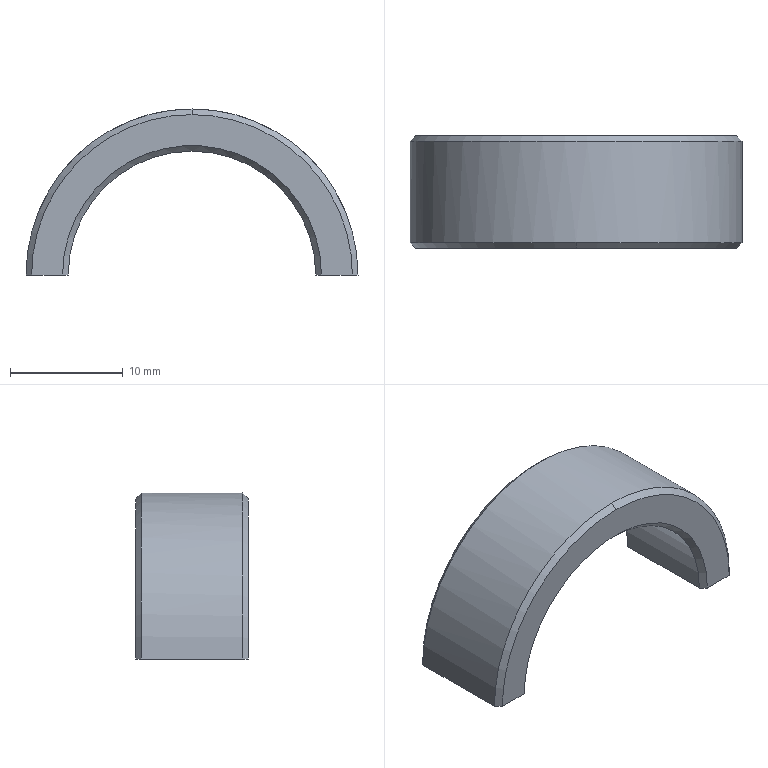Part | STEP file | Cuon T phu H01_3 | 1 solid | 12 faces | box 29.5 x 10 x 14.75 mm | volume 1497 mm3 | cone 6 | plane 4 | cylinder 2 | commonest cylinder face diameters 22 x1 29.5 x1
STEP:
#1=CARTESIAN_POINT('',(0.,0.,0.));
#2=DIRECTION('',(0.,0.,1.));
#3=DIRECTION('',(1.,0.,0.));
#4=AXIS2_PLACEMENT_3D('',#1,#2,#3);
#5=CARTESIAN_POINT('',(11.,9.5,0.));
#6=VERTEX_POINT('',#5);
#7=CARTESIAN_POINT('',(11.5,10.,0.));
#8=VERTEX_POINT('',#7);
#9=CARTESIAN_POINT('',(0.,-1.5,0.));
#10=DIRECTION('',(0.7071,0.7071,0.));
#11=VECTOR('',#10,1.);
#12=LINE('',#9,#11);
#13=CARTESIAN_POINT('',(0.,9.5,0.));
#14=DIRECTION('',(0.,1.,0.));
#15=DIRECTION('',(0.,0.,1.));
#16=AXIS2_PLACEMENT_3D('',#13,#14,#15);
#17=CONICAL_SURFACE('',#16,11.,0.7854);
#18=CARTESIAN_POINT('',(1.571,-11.));
#19=DIRECTION('',(0.,1.));
#20=VECTOR('',#19,1.);
#21=LINE('',#18,#20);
#22=(GEOMETRIC_REPRESENTATION_CONTEXT(2)PARAMETRIC_REPRESENTATION_CONTEXT()REPRESENTATION_CONTEXT('',''));
#23=DEFINITIONAL_REPRESENTATION('',(#21),#22);
#24=PCURVE('',#17,#23);
#25=CARTESIAN_POINT('',(120.,-52.57,0.));
#26=DIRECTION('',(0.,0.,1.));
#27=DIRECTION('',(1.,0.,0.));
#28=AXIS2_PLACEMENT_3D('',#25,#26,#27);
#29=PLANE('',#28);
#30=CARTESIAN_POINT('',(-120.,51.07));
#31=DIRECTION('',(0.7071,0.7071));
#32=VECTOR('',#31,1.);
#33=LINE('',#30,#32);
#34=(GEOMETRIC_REPRESENTATION_CONTEXT(2)PARAMETRIC_REPRESENTATION_CONTEXT()REPRESENTATION_CONTEXT('',''));
#35=DEFINITIONAL_REPRESENTATION('',(#33),#34);
#36=PCURVE('',#29,#35);
#37=SURFACE_CURVE('',#12,(#24,#36),.PCURVE_S1.);
#38=EDGE_CURVE('',#6,#8,#37,.T.);
#39=ORIENTED_EDGE('',*,*,#38,.T.);
#40=CARTESIAN_POINT('',(0.,10.,11.5));
#41=VERTEX_POINT('',#40);
#42=CARTESIAN_POINT('',(0.,10.,0.));
#43=DIRECTION('',(0.,-1.,0.));
#44=DIRECTION('',(0.,0.,1.));
#45=AXIS2_PLACEMENT_3D('',#42,#43,#44);
#46=CIRCLE('',#45,11.5);
#47=CARTESIAN_POINT('',(6.283,0.5));
#48=DIRECTION('',(-1.,0.));
#49=VECTOR('',#48,1.);
#50=LINE('',#47,#49);
#51=(GEOMETRIC_REPRESENTATION_CONTEXT(2)PARAMETRIC_REPRESENTATION_CONTEXT()REPRESENTATION_CONTEXT('',''));
#52=DEFINITIONAL_REPRESENTATION('',(#50),#51);
#53=PCURVE('',#17,#52);
#54=CARTESIAN_POINT('',(0.,10.,0.));
#55=DIRECTION('',(0.,1.,0.));
#56=DIRECTION('',(0.,0.,1.));
#57=AXIS2_PLACEMENT_3D('',#54,#55,#56);
#58=PLANE('',#57);
#59=CARTESIAN_POINT('',(11.5,0.));
#60=CARTESIAN_POINT('',(11.5,-19.919));
#61=CARTESIAN_POINT('',(-5.75,-9.959));
#62=CARTESIAN_POINT('',(-23.,0.));
#63=CARTESIAN_POINT('',(-5.75,9.959));
#64=CARTESIAN_POINT('',(11.5,19.919));
#65=CARTESIAN_POINT('',(11.5,0.));
#66=(BOUNDED_CURVE()B_SPLINE_CURVE(2,(#59,#60,#61,#62,#63,#64,#65),.UNSPECIFIED.,.T.,.F.)B_SPLINE_CURVE_WITH_KNOTS((1,2,2,2,2,1),(-2.094,0.,2.094,4.189,6.283,8.378),.UNSPECIFIED.)CURVE()GEOMETRIC_REPRESENTATION_ITEM()RATIONAL_B_SPLINE_CURVE((1.,0.5,1.,0.5,1.,0.5,1.))REPRESENTATION_ITEM(''));
#67=(GEOMETRIC_REPRESENTATION_CONTEXT(2)PARAMETRIC_REPRESENTATION_CONTEXT()REPRESENTATION_CONTEXT('',''));
#68=DEFINITIONAL_REPRESENTATION('',(#66),#67);
#69=PCURVE('',#58,#68);
#70=SURFACE_CURVE('',#46,(#53,#69),.PCURVE_S1.);
#71=EDGE_CURVE('',#8,#41,#70,.T.);
#72=ORIENTED_EDGE('',*,*,#71,.T.);
#73=CARTESIAN_POINT('',(0.,9.5,11.));
#74=VERTEX_POINT('',#73);
#75=CARTESIAN_POINT('',(0.,9.5,11.));
#76=DIRECTION('',(0.,0.7071,0.7071));
#77=VECTOR('',#76,1.);
#78=LINE('',#75,#77);
#79=CARTESIAN_POINT('',(0.,0.));
#80=DIRECTION('',(0.,1.));
#81=VECTOR('',#80,1.);
#82=LINE('',#79,#81);
#83=(GEOMETRIC_REPRESENTATION_CONTEXT(2)PARAMETRIC_REPRESENTATION_CONTEXT()REPRESENTATION_CONTEXT('',''));
#84=DEFINITIONAL_REPRESENTATION('',(#82),#83);
#85=PCURVE('',#17,#84);
#86=CARTESIAN_POINT('',(0.,9.5,0.));
#87=DIRECTION('',(0.,1.,0.));
#88=DIRECTION('',(0.,0.,1.));
#89=AXIS2_PLACEMENT_3D('',#86,#87,#88);
#90=CONICAL_SURFACE('',#89,11.,0.7854);
#91=CARTESIAN_POINT('',(6.283,0.));
#92=DIRECTION('',(0.,1.));
#93=VECTOR('',#92,1.);
#94=LINE('',#91,#93);
#95=(GEOMETRIC_REPRESENTATION_CONTEXT(2)PARAMETRIC_REPRESENTATION_CONTEXT()REPRESENTATION_CONTEXT('',''));
#96=DEFINITIONAL_REPRESENTATION('',(#94),#95);
#97=PCURVE('',#90,#96);
#98=SURFACE_CURVE('',#78,(#85,#97),.PCURVE_S1.);
#99=EDGE_CURVE('',#74,#41,#98,.T.);
#100=ORIENTED_EDGE('',*,*,#99,.F.);
#101=CARTESIAN_POINT('',(0.,9.5,0.));
#102=DIRECTION('',(0.,1.,0.));
#103=DIRECTION('',(0.,0.,1.));
#104=AXIS2_PLACEMENT_3D('',#101,#102,#103);
#105=CIRCLE('',#104,11.);
#106=CARTESIAN_POINT('',(0.,0.));
#107=DIRECTION('',(1.,0.));
#108=VECTOR('',#107,1.);
#109=LINE('',#106,#108);
#110=(GEOMETRIC_REPRESENTATION_CONTEXT(2)PARAMETRIC_REPRESENTATION_CONTEXT()REPRESENTATION_CONTEXT('',''));
#111=DEFINITIONAL_REPRESENTATION('',(#109),#110);
#112=PCURVE('',#17,#111);
#113=CARTESIAN_POINT('',(0.,10.,0.));
#114=DIRECTION('',(0.,-1.,0.));
#115=DIRECTION('',(0.,0.,-1.));
#116=AXIS2_PLACEMENT_3D('',#113,#114,#115);
#117=CYLINDRICAL_SURFACE('',#116,11.);
#118=CARTESIAN_POINT('',(3.142,0.5));
#119=DIRECTION('',(-1.,0.));
#120=VECTOR('',#119,1.);
#121=LINE('',#118,#120);
#122=(GEOMETRIC_REPRESENTATION_CONTEXT(2)PARAMETRIC_REPRESENTATION_CONTEXT()REPRESENTATION_CONTEXT('',''));
#123=DEFINITIONAL_REPRESENTATION('',(#121),#122);
#124=PCURVE('',#117,#123);
#125=SURFACE_CURVE('',#105,(#112,#124),.PCURVE_S1.);
#126=EDGE_CURVE('',#74,#6,#125,.T.);
#127=ORIENTED_EDGE('',*,*,#126,.T.);
#128=EDGE_LOOP('',(#39,#72,#100,#127));
#129=FACE_BOUND('',#128,.F.);
#130=ADVANCED_FACE('',(#129),#17,.F.);
#131=CARTESIAN_POINT('',(0.,0.,14.25));
#132=VERTEX_POINT('',#131);
#133=CARTESIAN_POINT('',(-14.25,0.,0.));
#134=VERTEX_POINT('',#133);
#135=CARTESIAN_POINT('',(0.,0.,0.));
#136=DIRECTION('',(0.,-1.,0.));
#137=DIRECTION('',(0.,0.,1.));
#138=AXIS2_PLACEMENT_3D('',#135,#136,#137);
#139=CIRCLE('',#138,14.25);
#140=CARTESIAN_POINT('',(0.,0.5,0.));
#141=DIRECTION('',(0.,1.,0.));
#142=DIRECTION('',(0.,0.,1.));
#143=AXIS2_PLACEMENT_3D('',#140,#141,#142);
#144=CONICAL_SURFACE('',#143,14.75,0.7854);
#145=CARTESIAN_POINT('',(6.283,-0.5));
#146=DIRECTION('',(-1.,0.));
#147=VECTOR('',#146,1.);
#148=LINE('',#145,#147);
#149=(GEOMETRIC_REPRESENTATION_CONTEXT(2)PARAMETRIC_REPRESENTATION_CONTEXT()REPRESENTATION_CONTEXT('',''));
#150=DEFINITIONAL_REPRESENTATION('',(#148),#149);
#151=PCURVE('',#144,#150);
#152=CARTESIAN_POINT('',(0.,0.,0.));
#153=DIRECTION('',(0.,1.,0.));
#154=DIRECTION('',(0.,0.,1.));
#155=AXIS2_PLACEMENT_3D('',#152,#153,#154);
#156=PLANE('',#155);
#157=CARTESIAN_POINT('',(14.25,0.));
#158=CARTESIAN_POINT('',(14.25,-24.682));
#159=CARTESIAN_POINT('',(-7.125,-12.341));
#160=CARTESIAN_POINT('',(-28.5,0.));
#161=CARTESIAN_POINT('',(-7.125,12.341));
#162=CARTESIAN_POINT('',(14.25,24.682));
#163=CARTESIAN_POINT('',(14.25,0.));
#164=(BOUNDED_CURVE()B_SPLINE_CURVE(2,(#157,#158,#159,#160,#161,#162,#163),.UNSPECIFIED.,.T.,.F.)B_SPLINE_CURVE_WITH_KNOTS((1,2,2,2,2,1),(-2.094,0.,2.094,4.189,6.283,8.378),.UNSPECIFIED.)CURVE()GEOMETRIC_REPRESENTATION_ITEM()RATIONAL_B_SPLINE_CURVE((1.,0.5,1.,0.5,1.,0.5,1.))REPRESENTATION_ITEM(''));
#165=(GEOMETRIC_REPRESENTATION_CONTEXT(2)PARAMETRIC_REPRESENTATION_CONTEXT()REPRESENTATION_CONTEXT('',''));
#166=DEFINITIONAL_REPRESENTATION('',(#164),#165);
#167=PCURVE('',#156,#166);
#168=SURFACE_CURVE('',#139,(#151,#167),.PCURVE_S1.);
#169=EDGE_CURVE('',#132,#134,#168,.T.);
#170=ORIENTED_EDGE('',*,*,#169,.F.);
#171=CARTESIAN_POINT('',(0.,0.5,14.75));
#172=VERTEX_POINT('',#171);
#173=CARTESIAN_POINT('',(0.,0.5,14.75));
#174=DIRECTION('',(0.,0.7071,0.7071));
#175=VECTOR('',#174,1.);
#176=LINE('',#173,#175);
#177=CARTESIAN_POINT('',(6.283,0.));
#178=DIRECTION('',(0.,1.));
#179=VECTOR('',#178,1.);
#180=LINE('',#177,#179);
#181=(GEOMETRIC_REPRESENTATION_CONTEXT(2)PARAMETRIC_REPRESENTATION_CONTEXT()REPRESENTATION_CONTEXT('',''));
#182=DEFINITIONAL_REPRESENTATION('',(#180),#181);
#183=PCURVE('',#144,#182);
#184=CARTESIAN_POINT('',(0.,0.5,0.));
#185=DIRECTION('',(0.,1.,0.));
#186=DIRECTION('',(0.,0.,1.));
#187=AXIS2_PLACEMENT_3D('',#184,#185,#186);
#188=CONICAL_SURFACE('',#187,14.75,0.7854);
#189=CARTESIAN_POINT('',(0.,0.));
#190=DIRECTION('',(0.,1.));
#191=VECTOR('',#190,1.);
#192=LINE('',#189,#191);
#193=(GEOMETRIC_REPRESENTATION_CONTEXT(2)PARAMETRIC_REPRESENTATION_CONTEXT()REPRESENTATION_CONTEXT('',''));
#194=DEFINITIONAL_REPRESENTATION('',(#192),#193);
#195=PCURVE('',#188,#194);
#196=SURFACE_CURVE('',#176,(#183,#195),.PCURVE_S1.);
#197=EDGE_CURVE('',#132,#172,#196,.T.);
#198=ORIENTED_EDGE('',*,*,#197,.T.);
#199=CARTESIAN_POINT('',(-14.75,0.5,0.));
#200=VERTEX_POINT('',#199);
#201=CARTESIAN_POINT('',(0.,0.5,0.));
#202=DIRECTION('',(0.,1.,0.));
#203=DIRECTION('',(0.,0.,1.));
#204=AXIS2_PLACEMENT_3D('',#201,#202,#203);
#205=CIRCLE('',#204,14.75);
#206=CARTESIAN_POINT('',(0.,0.));
#207=DIRECTION('',(1.,0.));
#208=VECTOR('',#207,1.);
#209=LINE('',#206,#208);
#210=(GEOMETRIC_REPRESENTATION_CONTEXT(2)PARAMETRIC_REPRESENTATION_CONTEXT()REPRESENTATION_CONTEXT('',''));
#211=DEFINITIONAL_REPRESENTATION('',(#209),#210);
#212=PCURVE('',#144,#211);
#213=CARTESIAN_POINT('',(0.,10.,0.));
#214=DIRECTION('',(0.,-1.,0.));
#215=DIRECTION('',(0.,0.,-1.));
#216=AXIS2_PLACEMENT_3D('',#213,#214,#215);
#217=CYLINDRICAL_SURFACE('',#216,14.75);
#218=CARTESIAN_POINT('',(9.425,9.5));
#219=DIRECTION('',(-1.,0.));
#220=VECTOR('',#219,1.);
#221=LINE('',#218,#220);
#222=(GEOMETRIC_REPRESENTATION_CONTEXT(2)PARAMETRIC_REPRESENTATION_CONTEXT()REPRESENTATION_CONTEXT('',''));
#223=DEFINITIONAL_REPRESENTATION('',(#221),#222);
#224=PCURVE('',#217,#223);
#225=SURFACE_CURVE('',#205,(#212,#224),.PCURVE_S1.);
#226=EDGE_CURVE('',#200,#172,#225,.T.);
#227=ORIENTED_EDGE('',*,*,#226,.F.);
#228=CARTESIAN_POINT('',(0.,-14.25,0.));
#229=DIRECTION('',(-0.7071,0.7071,0.));
#230=VECTOR('',#229,1.);
#231=LINE('',#228,#230);
#232=CARTESIAN_POINT('',(4.712,-14.75));
#233=DIRECTION('',(0.,1.));
#234=VECTOR('',#233,1.);
#235=LINE('',#232,#234);
#236=(GEOMETRIC_REPRESENTATION_CONTEXT(2)PARAMETRIC_REPRESENTATION_CONTEXT()REPRESENTATION_CONTEXT('',''));
#237=DEFINITIONAL_REPRESENTATION('',(#235),#236);
#238=PCURVE('',#144,#237);
#239=CARTESIAN_POINT('',(120.,-52.57,0.));
#240=DIRECTION('',(0.,0.,1.));
#241=DIRECTION('',(1.,0.,0.));
#242=AXIS2_PLACEMENT_3D('',#239,#240,#241);
#243=PLANE('',#242);
#244=CARTESIAN_POINT('',(-120.,38.32));
#245=DIRECTION('',(-0.7071,0.7071));
#246=VECTOR('',#245,1.);
#247=LINE('',#244,#246);
#248=(GEOMETRIC_REPRESENTATION_CONTEXT(2)PARAMETRIC_REPRESENTATION_CONTEXT()REPRESENTATION_CONTEXT('',''));
#249=DEFINITIONAL_REPRESENTATION('',(#247),#248);
#250=PCURVE('',#243,#249);
#251=SURFACE_CURVE('',#231,(#238,#250),.PCURVE_S1.);
#252=EDGE_CURVE('',#134,#200,#251,.T.);
#253=ORIENTED_EDGE('',*,*,#252,.F.);
#254=EDGE_LOOP('',(#170,#198,#227,#253));
#255=FACE_BOUND('',#254,.T.);
#256=ADVANCED_FACE('',(#255),#144,.T.);
#257=CARTESIAN_POINT('',(-14.25,10.,0.));
#258=VERTEX_POINT('',#257);
#259=CARTESIAN_POINT('',(-11.5,10.,0.));
#260=VERTEX_POINT('',#259);
#261=CARTESIAN_POINT('',(0.,10.,0.));
#262=DIRECTION('',(1.,0.,0.));
#263=VECTOR('',#262,1.);
#264=LINE('',#261,#263);
#265=CARTESIAN_POINT('',(0.,0.));
#266=DIRECTION('',(0.,1.));
#267=VECTOR('',#266,1.);
#268=LINE('',#265,#267);
#269=(GEOMETRIC_REPRESENTATION_CONTEXT(2)PARAMETRIC_REPRESENTATION_CONTEXT()REPRESENTATION_CONTEXT('',''));
#270=DEFINITIONAL_REPRESENTATION('',(#268),#269);
#271=PCURVE('',#58,#270);
#272=CARTESIAN_POINT('',(-120.,62.57));
#273=DIRECTION('',(1.,0.));
#274=VECTOR('',#273,1.);
#275=LINE('',#272,#274);
#276=(GEOMETRIC_REPRESENTATION_CONTEXT(2)PARAMETRIC_REPRESENTATION_CONTEXT()REPRESENTATION_CONTEXT('',''));
#277=DEFINITIONAL_REPRESENTATION('',(#275),#276);
#278=PCURVE('',#243,#277);
#279=SURFACE_CURVE('',#264,(#271,#278),.PCURVE_S1.);
#280=EDGE_CURVE('',#258,#260,#279,.T.);
#281=ORIENTED_EDGE('',*,*,#280,.F.);
#282=CARTESIAN_POINT('',(14.25,10.,0.));
#283=VERTEX_POINT('',#282);
#284=CARTESIAN_POINT('',(0.,10.,0.));
#285=DIRECTION('',(0.,1.,0.));
#286=DIRECTION('',(0.,0.,1.));
#287=AXIS2_PLACEMENT_3D('',#284,#285,#286);
#288=CIRCLE('',#287,14.25);
#289=CARTESIAN_POINT('',(0.,0.));
#290=DIRECTION('',(1.,0.));
#291=AXIS2_PLACEMENT_2D('',#289,#290);
#292=CIRCLE('',#291,14.25);
#293=(GEOMETRIC_REPRESENTATION_CONTEXT(2)PARAMETRIC_REPRESENTATION_CONTEXT()REPRESENTATION_CONTEXT('',''));
#294=DEFINITIONAL_REPRESENTATION('',(#292),#293);
#295=PCURVE('',#58,#294);
#296=CARTESIAN_POINT('',(0.,10.,0.));
#297=DIRECTION('',(0.,-1.,0.));
#298=DIRECTION('',(0.,0.,-1.));
#299=AXIS2_PLACEMENT_3D('',#296,#297,#298);
#300=CONICAL_SURFACE('',#299,14.25,0.7854);
#301=CARTESIAN_POINT('',(9.425,0.));
#302=DIRECTION('',(-1.,0.));
#303=VECTOR('',#302,1.);
#304=LINE('',#301,#303);
#305=(GEOMETRIC_REPRESENTATION_CONTEXT(2)PARAMETRIC_REPRESENTATION_CONTEXT()REPRESENTATION_CONTEXT('',''));
#306=DEFINITIONAL_REPRESENTATION('',(#304),#305);
#307=PCURVE('',#300,#306);
#308=SURFACE_CURVE('',#288,(#295,#307),.PCURVE_S1.);
#309=EDGE_CURVE('',#258,#283,#308,.T.);
#310=ORIENTED_EDGE('',*,*,#309,.T.);
#311=CARTESIAN_POINT('',(0.,10.,0.));
#312=DIRECTION('',(1.,0.,0.));
#313=VECTOR('',#312,1.);
#314=LINE('',#311,#313);
#315=CARTESIAN_POINT('',(0.,0.));
#316=DIRECTION('',(0.,1.));
#317=VECTOR('',#316,1.);
#318=LINE('',#315,#317);
#319=(GEOMETRIC_REPRESENTATION_CONTEXT(2)PARAMETRIC_REPRESENTATION_CONTEXT()REPRESENTATION_CONTEXT('',''));
#320=DEFINITIONAL_REPRESENTATION('',(#318),#319);
#321=PCURVE('',#58,#320);
#322=CARTESIAN_POINT('',(-120.,62.57));
#323=DIRECTION('',(1.,0.));
#324=VECTOR('',#323,1.);
#325=LINE('',#322,#324);
#326=(GEOMETRIC_REPRESENTATION_CONTEXT(2)PARAMETRIC_REPRESENTATION_CONTEXT()REPRESENTATION_CONTEXT('',''));
#327=DEFINITIONAL_REPRESENTATION('',(#325),#326);
#328=PCURVE('',#29,#327);
#329=SURFACE_CURVE('',#314,(#321,#328),.PCURVE_S1.);
#330=EDGE_CURVE('',#8,#283,#329,.T.);
#331=ORIENTED_EDGE('',*,*,#330,.F.);
#332=ORIENTED_EDGE('',*,*,#71,.T.);
#333=CARTESIAN_POINT('',(0.,10.,0.));
#334=DIRECTION('',(0.,-1.,0.));
#335=DIRECTION('',(0.,0.,1.));
#336=AXIS2_PLACEMENT_3D('',#333,#334,#335);
#337=CIRCLE('',#336,11.5);
#338=CARTESIAN_POINT('',(11.5,0.));
#339=CARTESIAN_POINT('',(11.5,-19.919));
#340=CARTESIAN_POINT('',(-5.75,-9.959));
#341=CARTESIAN_POINT('',(-23.,0.));
#342=CARTESIAN_POINT('',(-5.75,9.959));
#343=CARTESIAN_POINT('',(11.5,19.919));
#344=CARTESIAN_POINT('',(11.5,0.));
#345=(BOUNDED_CURVE()B_SPLINE_CURVE(2,(#338,#339,#340,#341,#342,#343,#344),.UNSPECIFIED.,.T.,.F.)B_SPLINE_CURVE_WITH_KNOTS((1,2,2,2,2,1),(-2.094,0.,2.094,4.189,6.283,8.378),.UNSPECIFIED.)CURVE()GEOMETRIC_REPRESENTATION_ITEM()RATIONAL_B_SPLINE_CURVE((1.,0.5,1.,0.5,1.,0.5,1.))REPRESENTATION_ITEM(''));
#346=(GEOMETRIC_REPRESENTATION_CONTEXT(2)PARAMETRIC_REPRESENTATION_CONTEXT()REPRESENTATION_CONTEXT('',''));
#347=DEFINITIONAL_REPRESENTATION('',(#345),#346);
#348=PCURVE('',#58,#347);
#349=CARTESIAN_POINT('',(6.283,0.5));
#350=DIRECTION('',(-1.,0.));
#351=VECTOR('',#350,1.);
#352=LINE('',#349,#351);
#353=(GEOMETRIC_REPRESENTATION_CONTEXT(2)PARAMETRIC_REPRESENTATION_CONTEXT()REPRESENTATION_CONTEXT('',''));
#354=DEFINITIONAL_REPRESENTATION('',(#352),#353);
#355=PCURVE('',#90,#354);
#356=SURFACE_CURVE('',#337,(#348,#355),.PCURVE_S1.);
#357=EDGE_CURVE('',#41,#260,#356,.T.);
#358=ORIENTED_EDGE('',*,*,#357,.T.);
#359=EDGE_LOOP('',(#281,#310,#331,#332,#358));
#360=FACE_BOUND('',#359,.T.);
#361=ADVANCED_FACE('',(#360),#58,.T.);
#362=CARTESIAN_POINT('',(14.25,0.,0.));
#363=VERTEX_POINT('',#362);
#364=CARTESIAN_POINT('',(0.,0.,0.));
#365=DIRECTION('',(0.,-1.,0.));
#366=DIRECTION('',(0.,0.,1.));
#367=AXIS2_PLACEMENT_3D('',#364,#365,#366);
#368=CIRCLE('',#367,14.25);
#369=CARTESIAN_POINT('',(14.25,0.));
#370=CARTESIAN_POINT('',(14.25,-24.682));
#371=CARTESIAN_POINT('',(-7.125,-12.341));
#372=CARTESIAN_POINT('',(-28.5,0.));
#373=CARTESIAN_POINT('',(-7.125,12.341));
#374=CARTESIAN_POINT('',(14.25,24.682));
#375=CARTESIAN_POINT('',(14.25,0.));
#376=(BOUNDED_CURVE()B_SPLINE_CURVE(2,(#369,#370,#371,#372,#373,#374,#375),.UNSPECIFIED.,.T.,.F.)B_SPLINE_CURVE_WITH_KNOTS((1,2,2,2,2,1),(-2.094,0.,2.094,4.189,6.283,8.378),.UNSPECIFIED.)CURVE()GEOMETRIC_REPRESENTATION_ITEM()RATIONAL_B_SPLINE_CURVE((1.,0.5,1.,0.5,1.,0.5,1.))REPRESENTATION_ITEM(''));
#377=(GEOMETRIC_REPRESENTATION_CONTEXT(2)PARAMETRIC_REPRESENTATION_CONTEXT()REPRESENTATION_CONTEXT('',''));
#378=DEFINITIONAL_REPRESENTATION('',(#376),#377);
#379=PCURVE('',#156,#378);
#380=CARTESIAN_POINT('',(6.283,-0.5));
#381=DIRECTION('',(-1.,0.));
#382=VECTOR('',#381,1.);
#383=LINE('',#380,#382);
#384=(GEOMETRIC_REPRESENTATION_CONTEXT(2)PARAMETRIC_REPRESENTATION_CONTEXT()REPRESENTATION_CONTEXT('',''));
#385=DEFINITIONAL_REPRESENTATION('',(#383),#384);
#386=PCURVE('',#188,#385);
#387=SURFACE_CURVE('',#368,(#379,#386),.PCURVE_S1.);
#388=EDGE_CURVE('',#363,#132,#387,.T.);
#389=ORIENTED_EDGE('',*,*,#388,.T.);
#390=ORIENTED_EDGE('',*,*,#169,.T.);
#391=CARTESIAN_POINT('',(-11.5,0.,0.));
#392=VERTEX_POINT('',#391);
#393=CARTESIAN_POINT('',(0.,0.,0.));
#394=DIRECTION('',(1.,0.,0.));
#395=VECTOR('',#394,1.);
#396=LINE('',#393,#395);
#397=CARTESIAN_POINT('',(0.,0.));
#398=DIRECTION('',(0.,1.));
#399=VECTOR('',#398,1.);
#400=LINE('',#397,#399);
#401=(GEOMETRIC_REPRESENTATION_CONTEXT(2)PARAMETRIC_REPRESENTATION_CONTEXT()REPRESENTATION_CONTEXT('',''));
#402=DEFINITIONAL_REPRESENTATION('',(#400),#401);
#403=PCURVE('',#156,#402);
#404=CARTESIAN_POINT('',(-120.,52.57));
#405=DIRECTION('',(1.,0.));
#406=VECTOR('',#405,1.);
#407=LINE('',#404,#406);
#408=(GEOMETRIC_REPRESENTATION_CONTEXT(2)PARAMETRIC_REPRESENTATION_CONTEXT()REPRESENTATION_CONTEXT('',''));
#409=DEFINITIONAL_REPRESENTATION('',(#407),#408);
#410=PCURVE('',#243,#409);
#411=SURFACE_CURVE('',#396,(#403,#410),.PCURVE_S1.);
#412=EDGE_CURVE('',#134,#392,#411,.T.);
#413=ORIENTED_EDGE('',*,*,#412,.T.);
#414=CARTESIAN_POINT('',(11.5,0.,0.));
#415=VERTEX_POINT('',#414);
#416=CARTESIAN_POINT('',(0.,0.,0.));
#417=DIRECTION('',(0.,1.,0.));
#418=DIRECTION('',(0.,0.,1.));
#419=AXIS2_PLACEMENT_3D('',#416,#417,#418);
#420=CIRCLE('',#419,11.5);
#421=CARTESIAN_POINT('',(0.,0.));
#422=DIRECTION('',(1.,0.));
#423=AXIS2_PLACEMENT_2D('',#421,#422);
#424=CIRCLE('',#423,11.5);
#425=(GEOMETRIC_REPRESENTATION_CONTEXT(2)PARAMETRIC_REPRESENTATION_CONTEXT()REPRESENTATION_CONTEXT('',''));
#426=DEFINITIONAL_REPRESENTATION('',(#424),#425);
#427=PCURVE('',#156,#426);
#428=CARTESIAN_POINT('',(0.,0.,0.));
#429=DIRECTION('',(0.,-1.,0.));
#430=DIRECTION('',(0.,0.,-1.));
#431=AXIS2_PLACEMENT_3D('',#428,#429,#430);
#432=CONICAL_SURFACE('',#431,11.5,0.7854);
#433=CARTESIAN_POINT('',(9.425,0.));
#434=DIRECTION('',(-1.,0.));
#435=VECTOR('',#434,1.);
#436=LINE('',#433,#435);
#437=(GEOMETRIC_REPRESENTATION_CONTEXT(2)PARAMETRIC_REPRESENTATION_CONTEXT()REPRESENTATION_CONTEXT('',''));
#438=DEFINITIONAL_REPRESENTATION('',(#436),#437);
#439=PCURVE('',#432,#438);
#440=SURFACE_CURVE('',#420,(#427,#439),.PCURVE_S1.);
#441=EDGE_CURVE('',#392,#415,#440,.T.);
#442=ORIENTED_EDGE('',*,*,#441,.T.);
#443=CARTESIAN_POINT('',(0.,0.,0.));
#444=DIRECTION('',(1.,0.,0.));
#445=VECTOR('',#444,1.);
#446=LINE('',#443,#445);
#447=CARTESIAN_POINT('',(0.,0.));
#448=DIRECTION('',(0.,1.));
#449=VECTOR('',#448,1.);
#450=LINE('',#447,#449);
#451=(GEOMETRIC_REPRESENTATION_CONTEXT(2)PARAMETRIC_REPRESENTATION_CONTEXT()REPRESENTATION_CONTEXT('',''));
#452=DEFINITIONAL_REPRESENTATION('',(#450),#451);
#453=PCURVE('',#156,#452);
#454=CARTESIAN_POINT('',(-120.,52.57));
#455=DIRECTION('',(1.,0.));
#456=VECTOR('',#455,1.);
#457=LINE('',#454,#456);
#458=(GEOMETRIC_REPRESENTATION_CONTEXT(2)PARAMETRIC_REPRESENTATION_CONTEXT()REPRESENTATION_CONTEXT('',''));
#459=DEFINITIONAL_REPRESENTATION('',(#457),#458);
#460=PCURVE('',#29,#459);
#461=SURFACE_CURVE('',#446,(#453,#460),.PCURVE_S1.);
#462=EDGE_CURVE('',#415,#363,#461,.T.);
#463=ORIENTED_EDGE('',*,*,#462,.T.);
#464=EDGE_LOOP('',(#389,#390,#413,#442,#463));
#465=FACE_BOUND('',#464,.T.);
#466=ADVANCED_FACE('',(#465),#156,.F.);
#467=CARTESIAN_POINT('',(14.75,9.5,0.));
#468=VERTEX_POINT('',#467);
#469=CARTESIAN_POINT('',(-14.75,9.5,0.));
#470=VERTEX_POINT('',#469);
#471=CARTESIAN_POINT('',(0.,9.5,0.));
#472=DIRECTION('',(0.,-1.,0.));
#473=DIRECTION('',(0.,0.,1.));
#474=AXIS2_PLACEMENT_3D('',#471,#472,#473);
#475=CIRCLE('',#474,14.75);
#476=CARTESIAN_POINT('',(-3.142,0.5));
#477=DIRECTION('',(1.,0.));
#478=VECTOR('',#477,1.);
#479=LINE('',#476,#478);
#480=(GEOMETRIC_REPRESENTATION_CONTEXT(2)PARAMETRIC_REPRESENTATION_CONTEXT()REPRESENTATION_CONTEXT('',''));
#481=DEFINITIONAL_REPRESENTATION('',(#479),#480);
#482=PCURVE('',#217,#481);
#483=CARTESIAN_POINT('',(-3.142,0.5));
#484=DIRECTION('',(1.,0.));
#485=VECTOR('',#484,1.);
#486=LINE('',#483,#485);
#487=(GEOMETRIC_REPRESENTATION_CONTEXT(2)PARAMETRIC_REPRESENTATION_CONTEXT()REPRESENTATION_CONTEXT('',''));
#488=DEFINITIONAL_REPRESENTATION('',(#486),#487);
#489=PCURVE('',#300,#488);
#490=SURFACE_CURVE('',#475,(#482,#489),.PCURVE_S1.);
#491=EDGE_CURVE('',#468,#470,#490,.T.);
#492=ORIENTED_EDGE('',*,*,#491,.T.);
#493=CARTESIAN_POINT('',(-14.75,10.,0.));
#494=DIRECTION('',(0.,-1.,0.));
#495=VECTOR('',#494,1.);
#496=LINE('',#493,#495);
#497=CARTESIAN_POINT('',(4.712,0.));
#498=DIRECTION('',(0.,1.));
#499=VECTOR('',#498,1.);
#500=LINE('',#497,#499);
#501=(GEOMETRIC_REPRESENTATION_CONTEXT(2)PARAMETRIC_REPRESENTATION_CONTEXT()REPRESENTATION_CONTEXT('',''));
#502=DEFINITIONAL_REPRESENTATION('',(#500),#501);
#503=PCURVE('',#217,#502);
#504=CARTESIAN_POINT('',(-134.75,62.57));
#505=DIRECTION('',(0.,-1.));
#506=VECTOR('',#505,1.);
#507=LINE('',#504,#506);
#508=(GEOMETRIC_REPRESENTATION_CONTEXT(2)PARAMETRIC_REPRESENTATION_CONTEXT()REPRESENTATION_CONTEXT('',''));
#509=DEFINITIONAL_REPRESENTATION('',(#507),#508);
#510=PCURVE('',#243,#509);
#511=SURFACE_CURVE('',#496,(#503,#510),.PCURVE_S1.);
#512=EDGE_CURVE('',#470,#200,#511,.T.);
#513=ORIENTED_EDGE('',*,*,#512,.T.);
#514=ORIENTED_EDGE('',*,*,#226,.T.);
#515=CARTESIAN_POINT('',(14.75,0.5,0.));
#516=VERTEX_POINT('',#515);
#517=CARTESIAN_POINT('',(0.,0.5,0.));
#518=DIRECTION('',(0.,1.,0.));
#519=DIRECTION('',(0.,0.,1.));
#520=AXIS2_PLACEMENT_3D('',#517,#518,#519);
#521=CIRCLE('',#520,14.75);
#522=CARTESIAN_POINT('',(3.142,9.5));
#523=DIRECTION('',(-1.,0.));
#524=VECTOR('',#523,1.);
#525=LINE('',#522,#524);
#526=(GEOMETRIC_REPRESENTATION_CONTEXT(2)PARAMETRIC_REPRESENTATION_CONTEXT()REPRESENTATION_CONTEXT('',''));
#527=DEFINITIONAL_REPRESENTATION('',(#525),#526);
#528=PCURVE('',#217,#527);
#529=CARTESIAN_POINT('',(0.,0.));
#530=DIRECTION('',(1.,0.));
#531=VECTOR('',#530,1.);
#532=LINE('',#529,#531);
#533=(GEOMETRIC_REPRESENTATION_CONTEXT(2)PARAMETRIC_REPRESENTATION_CONTEXT()REPRESENTATION_CONTEXT('',''));
#534=DEFINITIONAL_REPRESENTATION('',(#532),#533);
#535=PCURVE('',#188,#534);
#536=SURFACE_CURVE('',#521,(#528,#535),.PCURVE_S1.);
#537=EDGE_CURVE('',#172,#516,#536,.T.);
#538=ORIENTED_EDGE('',*,*,#537,.T.);
#539=CARTESIAN_POINT('',(14.75,10.,0.));
#540=DIRECTION('',(0.,1.,0.));
#541=VECTOR('',#540,1.);
#542=LINE('',#539,#541);
#543=CARTESIAN_POINT('',(1.571,0.));
#544=DIRECTION('',(0.,-1.));
#545=VECTOR('',#544,1.);
#546=LINE('',#543,#545);
#547=(GEOMETRIC_REPRESENTATION_CONTEXT(2)PARAMETRIC_REPRESENTATION_CONTEXT()REPRESENTATION_CONTEXT('',''));
#548=DEFINITIONAL_REPRESENTATION('',(#546),#547);
#549=PCURVE('',#217,#548);
#550=CARTESIAN_POINT('',(-105.25,62.57));
#551=DIRECTION('',(0.,1.));
#552=VECTOR('',#551,1.);
#553=LINE('',#550,#552);
#554=(GEOMETRIC_REPRESENTATION_CONTEXT(2)PARAMETRIC_REPRESENTATION_CONTEXT()REPRESENTATION_CONTEXT('',''));
#555=DEFINITIONAL_REPRESENTATION('',(#553),#554);
#556=PCURVE('',#29,#555);
#557=SURFACE_CURVE('',#542,(#549,#556),.PCURVE_S1.);
#558=EDGE_CURVE('',#516,#468,#557,.T.);
#559=ORIENTED_EDGE('',*,*,#558,.T.);
#560=EDGE_LOOP('',(#492,#513,#514,#538,#559));
#561=FACE_BOUND('',#560,.T.);
#562=ADVANCED_FACE('',(#561),#217,.T.);
#563=CARTESIAN_POINT('',(11.,0.5,0.));
#564=VERTEX_POINT('',#563);
#565=CARTESIAN_POINT('',(-11.,0.5,0.));
#566=VERTEX_POINT('',#565);
#567=CARTESIAN_POINT('',(0.,0.5,0.));
#568=DIRECTION('',(0.,-1.,0.));
#569=DIRECTION('',(0.,0.,1.));
#570=AXIS2_PLACEMENT_3D('',#567,#568,#569);
#571=CIRCLE('',#570,11.);
#572=CARTESIAN_POINT('',(-3.142,9.5));
#573=DIRECTION('',(1.,0.));
#574=VECTOR('',#573,1.);
#575=LINE('',#572,#574);
#576=(GEOMETRIC_REPRESENTATION_CONTEXT(2)PARAMETRIC_REPRESENTATION_CONTEXT()REPRESENTATION_CONTEXT('',''));
#577=DEFINITIONAL_REPRESENTATION('',(#575),#576);
#578=PCURVE('',#117,#577);
#579=CARTESIAN_POINT('',(-3.142,-0.5));
#580=DIRECTION('',(1.,0.));
#581=VECTOR('',#580,1.);
#582=LINE('',#579,#581);
#583=(GEOMETRIC_REPRESENTATION_CONTEXT(2)PARAMETRIC_REPRESENTATION_CONTEXT()REPRESENTATION_CONTEXT('',''));
#584=DEFINITIONAL_REPRESENTATION('',(#582),#583);
#585=PCURVE('',#432,#584);
#586=SURFACE_CURVE('',#571,(#578,#585),.PCURVE_S1.);
#587=EDGE_CURVE('',#564,#566,#586,.T.);
#588=ORIENTED_EDGE('',*,*,#587,.F.);
#589=CARTESIAN_POINT('',(11.,10.,0.));
#590=DIRECTION('',(0.,1.,0.));
#591=VECTOR('',#590,1.);
#592=LINE('',#589,#591);
#593=CARTESIAN_POINT('',(1.571,0.));
#594=DIRECTION('',(0.,-1.));
#595=VECTOR('',#594,1.);
#596=LINE('',#593,#595);
#597=(GEOMETRIC_REPRESENTATION_CONTEXT(2)PARAMETRIC_REPRESENTATION_CONTEXT()REPRESENTATION_CONTEXT('',''));
#598=DEFINITIONAL_REPRESENTATION('',(#596),#597);
#599=PCURVE('',#117,#598);
#600=CARTESIAN_POINT('',(-109.,62.57));
#601=DIRECTION('',(0.,1.));
#602=VECTOR('',#601,1.);
#603=LINE('',#600,#602);
#604=(GEOMETRIC_REPRESENTATION_CONTEXT(2)PARAMETRIC_REPRESENTATION_CONTEXT()REPRESENTATION_CONTEXT('',''));
#605=DEFINITIONAL_REPRESENTATION('',(#603),#604);
#606=PCURVE('',#29,#605);
#607=SURFACE_CURVE('',#592,(#599,#606),.PCURVE_S1.);
#608=EDGE_CURVE('',#564,#6,#607,.T.);
#609=ORIENTED_EDGE('',*,*,#608,.T.);
#610=ORIENTED_EDGE('',*,*,#126,.F.);
#611=CARTESIAN_POINT('',(-11.,9.5,0.));
#612=VERTEX_POINT('',#611);
#613=CARTESIAN_POINT('',(0.,9.5,0.));
#614=DIRECTION('',(0.,1.,0.));
#615=DIRECTION('',(0.,0.,1.));
#616=AXIS2_PLACEMENT_3D('',#613,#614,#615);
#617=CIRCLE('',#616,11.);
#618=CARTESIAN_POINT('',(9.425,0.5));
#619=DIRECTION('',(-1.,0.));
#620=VECTOR('',#619,1.);
#621=LINE('',#618,#620);
#622=(GEOMETRIC_REPRESENTATION_CONTEXT(2)PARAMETRIC_REPRESENTATION_CONTEXT()REPRESENTATION_CONTEXT('',''));
#623=DEFINITIONAL_REPRESENTATION('',(#621),#622);
#624=PCURVE('',#117,#623);
#625=CARTESIAN_POINT('',(0.,0.));
#626=DIRECTION('',(1.,0.));
#627=VECTOR('',#626,1.);
#628=LINE('',#625,#627);
#629=(GEOMETRIC_REPRESENTATION_CONTEXT(2)PARAMETRIC_REPRESENTATION_CONTEXT()REPRESENTATION_CONTEXT('',''));
#630=DEFINITIONAL_REPRESENTATION('',(#628),#629);
#631=PCURVE('',#90,#630);
#632=SURFACE_CURVE('',#617,(#624,#631),.PCURVE_S1.);
#633=EDGE_CURVE('',#612,#74,#632,.T.);
#634=ORIENTED_EDGE('',*,*,#633,.F.);
#635=CARTESIAN_POINT('',(-11.,10.,0.));
#636=DIRECTION('',(0.,-1.,0.));
#637=VECTOR('',#636,1.);
#638=LINE('',#635,#637);
#639=CARTESIAN_POINT('',(4.712,0.));
#640=DIRECTION('',(0.,1.));
#641=VECTOR('',#640,1.);
#642=LINE('',#639,#641);
#643=(GEOMETRIC_REPRESENTATION_CONTEXT(2)PARAMETRIC_REPRESENTATION_CONTEXT()REPRESENTATION_CONTEXT('',''));
#644=DEFINITIONAL_REPRESENTATION('',(#642),#643);
#645=PCURVE('',#117,#644);
#646=CARTESIAN_POINT('',(-131.,62.57));
#647=DIRECTION('',(0.,-1.));
#648=VECTOR('',#647,1.);
#649=LINE('',#646,#648);
#650=(GEOMETRIC_REPRESENTATION_CONTEXT(2)PARAMETRIC_REPRESENTATION_CONTEXT()REPRESENTATION_CONTEXT('',''));
#651=DEFINITIONAL_REPRESENTATION('',(#649),#650);
#652=PCURVE('',#243,#651);
#653=SURFACE_CURVE('',#638,(#645,#652),.PCURVE_S1.);
#654=EDGE_CURVE('',#612,#566,#653,.T.);
#655=ORIENTED_EDGE('',*,*,#654,.T.);
#656=EDGE_LOOP('',(#588,#609,#610,#634,#655));
#657=FACE_BOUND('',#656,.F.);
#658=ADVANCED_FACE('',(#657),#117,.F.);
#659=ORIENTED_EDGE('',*,*,#197,.F.);
#660=ORIENTED_EDGE('',*,*,#388,.F.);
#661=CARTESIAN_POINT('',(0.,-14.25,0.));
#662=DIRECTION('',(-0.7071,-0.7071,0.));
#663=VECTOR('',#662,1.);
#664=LINE('',#661,#663);
#665=CARTESIAN_POINT('',(1.571,-14.75));
#666=DIRECTION('',(0.,-1.));
#667=VECTOR('',#666,1.);
#668=LINE('',#665,#667);
#669=(GEOMETRIC_REPRESENTATION_CONTEXT(2)PARAMETRIC_REPRESENTATION_CONTEXT()REPRESENTATION_CONTEXT('',''));
#670=DEFINITIONAL_REPRESENTATION('',(#668),#669);
#671=PCURVE('',#188,#670);
#672=CARTESIAN_POINT('',(-120.,38.32));
#673=DIRECTION('',(-0.7071,-0.7071));
#674=VECTOR('',#673,1.);
#675=LINE('',#672,#674);
#676=(GEOMETRIC_REPRESENTATION_CONTEXT(2)PARAMETRIC_REPRESENTATION_CONTEXT()REPRESENTATION_CONTEXT('',''));
#677=DEFINITIONAL_REPRESENTATION('',(#675),#676);
#678=PCURVE('',#29,#677);
#679=SURFACE_CURVE('',#664,(#671,#678),.PCURVE_S1.);
#680=EDGE_CURVE('',#516,#363,#679,.T.);
#681=ORIENTED_EDGE('',*,*,#680,.F.);
#682=ORIENTED_EDGE('',*,*,#537,.F.);
#683=EDGE_LOOP('',(#659,#660,#681,#682));
#684=FACE_BOUND('',#683,.T.);
#685=ADVANCED_FACE('',(#684),#188,.T.);
#686=CARTESIAN_POINT('',(0.,24.25,0.));
#687=DIRECTION('',(0.7071,0.7071,0.));
#688=VECTOR('',#687,1.);
#689=LINE('',#686,#688);
#690=CARTESIAN_POINT('',(4.712,-14.25));
#691=DIRECTION('',(0.,-1.));
#692=VECTOR('',#691,1.);
#693=LINE('',#690,#692);
#694=(GEOMETRIC_REPRESENTATION_CONTEXT(2)PARAMETRIC_REPRESENTATION_CONTEXT()REPRESENTATION_CONTEXT('',''));
#695=DEFINITIONAL_REPRESENTATION('',(#693),#694);
#696=PCURVE('',#300,#695);
#697=CARTESIAN_POINT('',(-120.,76.82));
#698=DIRECTION('',(0.7071,0.7071));
#699=VECTOR('',#698,1.);
#700=LINE('',#697,#699);
#701=(GEOMETRIC_REPRESENTATION_CONTEXT(2)PARAMETRIC_REPRESENTATION_CONTEXT()REPRESENTATION_CONTEXT('',''));
#702=DEFINITIONAL_REPRESENTATION('',(#700),#701);
#703=PCURVE('',#243,#702);
#704=SURFACE_CURVE('',#689,(#696,#703),.PCURVE_S1.);
#705=EDGE_CURVE('',#470,#258,#704,.T.);
#706=ORIENTED_EDGE('',*,*,#705,.F.);
#707=ORIENTED_EDGE('',*,*,#491,.F.);
#708=CARTESIAN_POINT('',(0.,24.25,0.));
#709=DIRECTION('',(0.7071,-0.7071,0.));
#710=VECTOR('',#709,1.);
#711=LINE('',#708,#710);
#712=CARTESIAN_POINT('',(1.571,-14.25));
#713=DIRECTION('',(0.,1.));
#714=VECTOR('',#713,1.);
#715=LINE('',#712,#714);
#716=(GEOMETRIC_REPRESENTATION_CONTEXT(2)PARAMETRIC_REPRESENTATION_CONTEXT()REPRESENTATION_CONTEXT('',''));
#717=DEFINITIONAL_REPRESENTATION('',(#715),#716);
#718=PCURVE('',#300,#717);
#719=CARTESIAN_POINT('',(-120.,76.82));
#720=DIRECTION('',(0.7071,-0.7071));
#721=VECTOR('',#720,1.);
#722=LINE('',#719,#721);
#723=(GEOMETRIC_REPRESENTATION_CONTEXT(2)PARAMETRIC_REPRESENTATION_CONTEXT()REPRESENTATION_CONTEXT('',''));
#724=DEFINITIONAL_REPRESENTATION('',(#722),#723);
#725=PCURVE('',#29,#724);
#726=SURFACE_CURVE('',#711,(#718,#725),.PCURVE_S1.);
#727=EDGE_CURVE('',#283,#468,#726,.T.);
#728=ORIENTED_EDGE('',*,*,#727,.F.);
#729=ORIENTED_EDGE('',*,*,#309,.F.);
#730=EDGE_LOOP('',(#706,#707,#728,#729));
#731=FACE_BOUND('',#730,.T.);
#732=ADVANCED_FACE('',(#731),#300,.T.);
#733=ORIENTED_EDGE('',*,*,#441,.T.);
#734=CARTESIAN_POINT('',(0.,11.5,0.));
#735=DIRECTION('',(-0.7071,0.7071,0.));
#736=VECTOR('',#735,1.);
#737=LINE('',#734,#736);
#738=CARTESIAN_POINT('',(1.571,-11.5));
#739=DIRECTION('',(0.,-1.));
#740=VECTOR('',#739,1.);
#741=LINE('',#738,#740);
#742=(GEOMETRIC_REPRESENTATION_CONTEXT(2)PARAMETRIC_REPRESENTATION_CONTEXT()REPRESENTATION_CONTEXT('',''));
#743=DEFINITIONAL_REPRESENTATION('',(#741),#742);
#744=PCURVE('',#432,#743);
#745=CARTESIAN_POINT('',(-120.,64.07));
#746=DIRECTION('',(-0.7071,0.7071));
#747=VECTOR('',#746,1.);
#748=LINE('',#745,#747);
#749=(GEOMETRIC_REPRESENTATION_CONTEXT(2)PARAMETRIC_REPRESENTATION_CONTEXT()REPRESENTATION_CONTEXT('',''));
#750=DEFINITIONAL_REPRESENTATION('',(#748),#749);
#751=PCURVE('',#29,#750);
#752=SURFACE_CURVE('',#737,(#744,#751),.PCURVE_S1.);
#753=EDGE_CURVE('',#415,#564,#752,.T.);
#754=ORIENTED_EDGE('',*,*,#753,.T.);
#755=ORIENTED_EDGE('',*,*,#587,.T.);
#756=CARTESIAN_POINT('',(0.,11.5,0.));
#757=DIRECTION('',(-0.7071,-0.7071,0.));
#758=VECTOR('',#757,1.);
#759=LINE('',#756,#758);
#760=CARTESIAN_POINT('',(4.712,-11.5));
#761=DIRECTION('',(0.,1.));
#762=VECTOR('',#761,1.);
#763=LINE('',#760,#762);
#764=(GEOMETRIC_REPRESENTATION_CONTEXT(2)PARAMETRIC_REPRESENTATION_CONTEXT()REPRESENTATION_CONTEXT('',''));
#765=DEFINITIONAL_REPRESENTATION('',(#763),#764);
#766=PCURVE('',#432,#765);
#767=CARTESIAN_POINT('',(-120.,64.07));
#768=DIRECTION('',(-0.7071,-0.7071));
#769=VECTOR('',#768,1.);
#770=LINE('',#767,#769);
#771=(GEOMETRIC_REPRESENTATION_CONTEXT(2)PARAMETRIC_REPRESENTATION_CONTEXT()REPRESENTATION_CONTEXT('',''));
#772=DEFINITIONAL_REPRESENTATION('',(#770),#771);
#773=PCURVE('',#243,#772);
#774=SURFACE_CURVE('',#759,(#766,#773),.PCURVE_S1.);
#775=EDGE_CURVE('',#566,#392,#774,.T.);
#776=ORIENTED_EDGE('',*,*,#775,.T.);
#777=EDGE_LOOP('',(#733,#754,#755,#776));
#778=FACE_BOUND('',#777,.F.);
#779=ADVANCED_FACE('',(#778),#432,.F.);
#780=ORIENTED_EDGE('',*,*,#357,.T.);
#781=CARTESIAN_POINT('',(0.,-1.5,0.));
#782=DIRECTION('',(0.7071,-0.7071,0.));
#783=VECTOR('',#782,1.);
#784=LINE('',#781,#783);
#785=CARTESIAN_POINT('',(4.712,-11.));
#786=DIRECTION('',(0.,-1.));
#787=VECTOR('',#786,1.);
#788=LINE('',#785,#787);
#789=(GEOMETRIC_REPRESENTATION_CONTEXT(2)PARAMETRIC_REPRESENTATION_CONTEXT()REPRESENTATION_CONTEXT('',''));
#790=DEFINITIONAL_REPRESENTATION('',(#788),#789);
#791=PCURVE('',#90,#790);
#792=CARTESIAN_POINT('',(-120.,51.07));
#793=DIRECTION('',(0.7071,-0.7071));
#794=VECTOR('',#793,1.);
#795=LINE('',#792,#794);
#796=(GEOMETRIC_REPRESENTATION_CONTEXT(2)PARAMETRIC_REPRESENTATION_CONTEXT()REPRESENTATION_CONTEXT('',''));
#797=DEFINITIONAL_REPRESENTATION('',(#795),#796);
#798=PCURVE('',#243,#797);
#799=SURFACE_CURVE('',#784,(#791,#798),.PCURVE_S1.);
#800=EDGE_CURVE('',#260,#612,#799,.T.);
#801=ORIENTED_EDGE('',*,*,#800,.T.);
#802=ORIENTED_EDGE('',*,*,#633,.T.);
#803=ORIENTED_EDGE('',*,*,#99,.T.);
#804=EDGE_LOOP('',(#780,#801,#802,#803));
#805=FACE_BOUND('',#804,.F.);
#806=ADVANCED_FACE('',(#805),#90,.F.);
#807=ORIENTED_EDGE('',*,*,#252,.T.);
#808=ORIENTED_EDGE('',*,*,#512,.F.);
#809=ORIENTED_EDGE('',*,*,#705,.T.);
#810=ORIENTED_EDGE('',*,*,#280,.T.);
#811=ORIENTED_EDGE('',*,*,#800,.T.);
#812=ORIENTED_EDGE('',*,*,#654,.T.);
#813=ORIENTED_EDGE('',*,*,#775,.T.);
#814=ORIENTED_EDGE('',*,*,#412,.F.);
#815=EDGE_LOOP('',(#807,#808,#809,#810,#811,#812,#813,#814));
#816=FACE_BOUND('',#815,.T.);
#817=ADVANCED_FACE('',(#816),#243,.F.);
#818=ORIENTED_EDGE('',*,*,#680,.T.);
#819=ORIENTED_EDGE('',*,*,#462,.F.);
#820=ORIENTED_EDGE('',*,*,#753,.T.);
#821=ORIENTED_EDGE('',*,*,#608,.T.);
#822=ORIENTED_EDGE('',*,*,#38,.T.);
#823=ORIENTED_EDGE('',*,*,#330,.T.);
#824=ORIENTED_EDGE('',*,*,#727,.T.);
#825=ORIENTED_EDGE('',*,*,#558,.F.);
#826=EDGE_LOOP('',(#818,#819,#820,#821,#822,#823,#824,#825));
#827=FACE_BOUND('',#826,.T.);
#828=ADVANCED_FACE('',(#827),#29,.F.);
#829=CLOSED_SHELL('',(#130,#256,#361,#466,#562,#658,#685,#732,#779,#806,#817,#828));
#830=MANIFOLD_SOLID_BREP('',#829);
#831=(LENGTH_UNIT()NAMED_UNIT(*)SI_UNIT(.MILLI.,.METRE.));
#832=UNCERTAINTY_MEASURE_WITH_UNIT(LENGTH_MEASURE(0.0000001),#831,'','');
#833=(NAMED_UNIT(*)PLANE_ANGLE_UNIT()SI_UNIT($,.RADIAN.));
#834=(NAMED_UNIT(*)SI_UNIT($,.STERADIAN.)SOLID_ANGLE_UNIT());
#835=(GEOMETRIC_REPRESENTATION_CONTEXT(3)GLOBAL_UNCERTAINTY_ASSIGNED_CONTEXT((#832))GLOBAL_UNIT_ASSIGNED_CONTEXT((#831,#833,#834))REPRESENTATION_CONTEXT('',''));
#836=ADVANCED_BREP_SHAPE_REPRESENTATION('',(#4,#830),#835);